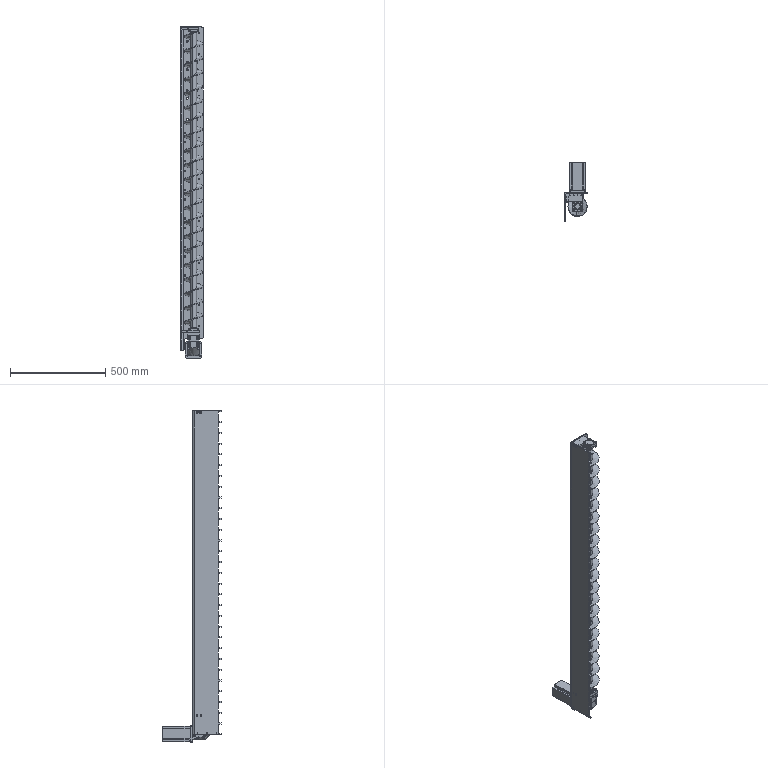Part | SolidWorks | features CompositeCurve 2 | 27 solids | 1291 faces | box 120 x 307 x 1742 mm | volume 4964407 mm3 | cylinder 594 | plane 471 | cone 133 | spline 53 | torus 40 | commonest cylinder face diameters 4.2 x94 6.8 x64 5.8 x54 10 x52 69 x26 3.3 x18